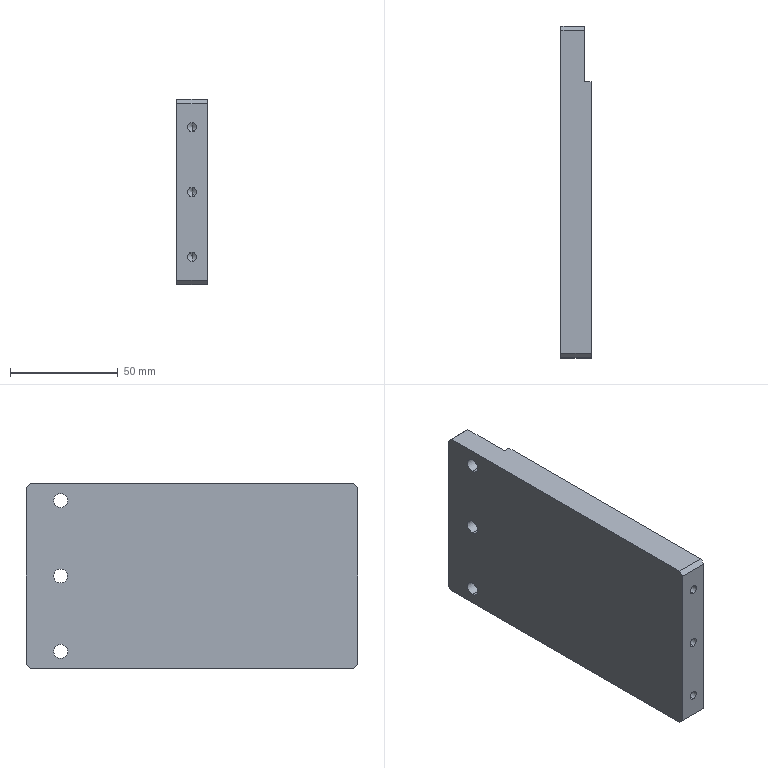Part | STEP file | 1 solid | 30 faces | box 14 x 154 x 86 mm | volume 176980 mm3 | cylinder 12 | plane 12 | cone 6 | commonest cylinder face diameters 4.2 x6 6.5 x6